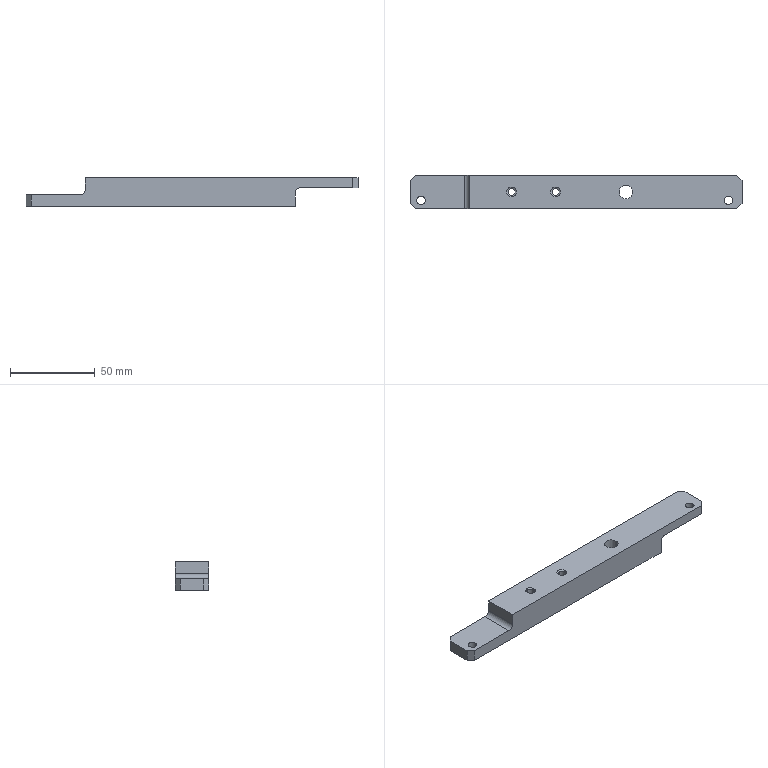Part | NX | 1 solid | 34 faces | box 196 x 20 x 17 mm | volume 49787 mm3 | plane 14 | cylinder 14 | cone 6 | commonest cylinder face diameters 4.2 x6 5 x4 6 x2 8 x2
STEP:
#1=CARTESIAN_POINT('',(-95.,10.,-1.5));
#2=VERTEX_POINT('',#1);
#3=CARTESIAN_POINT('',(-66.,10.,-1.5));
#4=VERTEX_POINT('',#3);
#5=CARTESIAN_POINT('',(0.,10.,-1.5));
#6=DIRECTION('',(1.,0.,0.));
#7=VECTOR('',#6,1000.);
#8=LINE('',#5,#7);
#9=EDGE_CURVE('',#2,#4,#8,.T.);
#10=ORIENTED_EDGE('',*,*,#9,.F.);
#11=CARTESIAN_POINT('',(-98.,7.,-1.5));
#12=VERTEX_POINT('',#11);
#13=CARTESIAN_POINT('',(-95.,10.,-1.5));
#14=DIRECTION('',(-0.7071,-0.7071,0.));
#15=VECTOR('',#14,1000.);
#16=LINE('',#13,#15);
#17=EDGE_CURVE('',#2,#12,#16,.T.);
#18=ORIENTED_EDGE('',*,*,#17,.T.);
#19=CARTESIAN_POINT('',(-98.,-7.,-1.5));
#20=VERTEX_POINT('',#19);
#21=CARTESIAN_POINT('',(-98.,-7.,-1.5));
#22=DIRECTION('',(0.,1.,0.));
#23=VECTOR('',#22,1000.);
#24=LINE('',#21,#23);
#25=EDGE_CURVE('',#20,#12,#24,.T.);
#26=ORIENTED_EDGE('',*,*,#25,.F.);
#27=CARTESIAN_POINT('',(-95.,-10.,-1.5));
#28=VERTEX_POINT('',#27);
#29=CARTESIAN_POINT('',(-98.,-7.,-1.5));
#30=DIRECTION('',(0.7071,-0.7071,0.));
#31=VECTOR('',#30,1000.);
#32=LINE('',#29,#31);
#33=EDGE_CURVE('',#20,#28,#32,.T.);
#34=ORIENTED_EDGE('',*,*,#33,.T.);
#35=CARTESIAN_POINT('',(-66.,-10.,-1.5));
#36=VERTEX_POINT('',#35);
#37=CARTESIAN_POINT('',(-66.,-10.,-1.5));
#38=DIRECTION('',(-1.,0.,0.));
#39=VECTOR('',#38,1000.);
#40=LINE('',#37,#39);
#41=EDGE_CURVE('',#36,#28,#40,.T.);
#42=ORIENTED_EDGE('',*,*,#41,.F.);
#43=CARTESIAN_POINT('',(-66.,10.,-1.5));
#44=DIRECTION('',(0.,-1.,0.));
#45=VECTOR('',#44,1000.);
#46=LINE('',#43,#45);
#47=EDGE_CURVE('',#4,#36,#46,.T.);
#48=ORIENTED_EDGE('',*,*,#47,.F.);
#49=EDGE_LOOP('',(#10,#18,#26,#34,#42,#48));
#50=FACE_BOUND('',#49,.T.);
#51=CARTESIAN_POINT('',(-94.,-5.,-1.5));
#52=VERTEX_POINT('',#51);
#53=CARTESIAN_POINT('',(-89.,-5.,-1.5));
#54=VERTEX_POINT('',#53);
#55=CARTESIAN_POINT('',(-91.5,-5.,-1.5));
#56=DIRECTION('',(0.,0.,-1.));
#57=DIRECTION('',(-1.,0.,0.));
#58=AXIS2_PLACEMENT_3D('',#55,#56,#57);
#59=CIRCLE('',#58,2.5);
#60=EDGE_CURVE('',#52,#54,#59,.T.);
#61=ORIENTED_EDGE('',*,*,#60,.T.);
#62=CARTESIAN_POINT('',(-91.5,-5.,-1.5));
#63=DIRECTION('',(0.,0.,-1.));
#64=DIRECTION('',(-1.,0.,0.));
#65=AXIS2_PLACEMENT_3D('',#62,#63,#64);
#66=CIRCLE('',#65,2.5);
#67=EDGE_CURVE('',#54,#52,#66,.T.);
#68=ORIENTED_EDGE('',*,*,#67,.T.);
#69=EDGE_LOOP('',(#61,#68));
#70=FACE_BOUND('',#69,.T.);
#71=CARTESIAN_POINT('',(-98.,10.,-1.5));
#72=DIRECTION('',(0.,0.,1.));
#73=DIRECTION('',(1.,0.,0.));
#74=AXIS2_PLACEMENT_3D('',#71,#72,#73);
#75=PLANE('',#74);
#76=ADVANCED_FACE('',(#50,#70),#75,.T.);
#77=CARTESIAN_POINT('',(61.,-10.,-0.5));
#78=VERTEX_POINT('',#77);
#79=CARTESIAN_POINT('',(64.,-10.,2.5));
#80=VERTEX_POINT('',#79);
#81=CARTESIAN_POINT('',(64.,-10.,-0.5));
#82=DIRECTION('',(0.,1.,0.));
#83=DIRECTION('',(-1.,0.,0.));
#84=AXIS2_PLACEMENT_3D('',#81,#82,#83);
#85=CIRCLE('',#84,3.);
#86=EDGE_CURVE('',#78,#80,#85,.T.);
#87=ORIENTED_EDGE('',*,*,#86,.T.);
#88=CARTESIAN_POINT('',(95.,-10.,2.5));
#89=VERTEX_POINT('',#88);
#90=CARTESIAN_POINT('',(64.,-10.,2.5));
#91=DIRECTION('',(1.,0.,0.));
#92=VECTOR('',#91,1000.);
#93=LINE('',#90,#92);
#94=EDGE_CURVE('',#80,#89,#93,.T.);
#95=ORIENTED_EDGE('',*,*,#94,.T.);
#96=CARTESIAN_POINT('',(95.,-10.,8.5));
#97=VERTEX_POINT('',#96);
#98=CARTESIAN_POINT('',(95.,-10.,2.5));
#99=DIRECTION('',(0.,0.,1.));
#100=VECTOR('',#99,1000.);
#101=LINE('',#98,#100);
#102=EDGE_CURVE('',#89,#97,#101,.T.);
#103=ORIENTED_EDGE('',*,*,#102,.T.);
#104=CARTESIAN_POINT('',(-63.,-10.,8.5));
#105=VERTEX_POINT('',#104);
#106=CARTESIAN_POINT('',(0.,-10.,8.5));
#107=DIRECTION('',(1.,0.,0.));
#108=VECTOR('',#107,1000.);
#109=LINE('',#106,#108);
#110=EDGE_CURVE('',#105,#97,#109,.T.);
#111=ORIENTED_EDGE('',*,*,#110,.F.);
#112=CARTESIAN_POINT('',(-63.,-10.,1.5));
#113=VERTEX_POINT('',#112);
#114=CARTESIAN_POINT('',(-63.,-10.,1.5));
#115=DIRECTION('',(0.,0.,1.));
#116=VECTOR('',#115,1000.);
#117=LINE('',#114,#116);
#118=EDGE_CURVE('',#113,#105,#117,.T.);
#119=ORIENTED_EDGE('',*,*,#118,.F.);
#120=CARTESIAN_POINT('',(-66.,-10.,1.5));
#121=DIRECTION('',(0.,1.,0.));
#122=DIRECTION('',(1.,0.,0.));
#123=AXIS2_PLACEMENT_3D('',#120,#121,#122);
#124=CIRCLE('',#123,3.);
#125=EDGE_CURVE('',#113,#36,#124,.T.);
#126=ORIENTED_EDGE('',*,*,#125,.T.);
#127=ORIENTED_EDGE('',*,*,#41,.T.);
#128=CARTESIAN_POINT('',(-95.,-10.,-8.5));
#129=VERTEX_POINT('',#128);
#130=CARTESIAN_POINT('',(-95.,-10.,-8.5));
#131=DIRECTION('',(0.,0.,1.));
#132=VECTOR('',#131,1000.);
#133=LINE('',#130,#132);
#134=EDGE_CURVE('',#129,#28,#133,.T.);
#135=ORIENTED_EDGE('',*,*,#134,.F.);
#136=CARTESIAN_POINT('',(61.,-10.,-8.5));
#137=VERTEX_POINT('',#136);
#138=CARTESIAN_POINT('',(0.,-10.,-8.5));
#139=DIRECTION('',(1.,0.,0.));
#140=VECTOR('',#139,1000.);
#141=LINE('',#138,#140);
#142=EDGE_CURVE('',#129,#137,#141,.T.);
#143=ORIENTED_EDGE('',*,*,#142,.T.);
#144=CARTESIAN_POINT('',(61.,-10.,-0.5));
#145=DIRECTION('',(0.,0.,-1.));
#146=VECTOR('',#145,1000.);
#147=LINE('',#144,#146);
#148=EDGE_CURVE('',#78,#137,#147,.T.);
#149=ORIENTED_EDGE('',*,*,#148,.F.);
#150=EDGE_LOOP('',(#87,#95,#103,#111,#119,#126,#127,#135,#143,#149));
#151=FACE_BOUND('',#150,.T.);
#152=CARTESIAN_POINT('',(-98.,-10.,8.5));
#153=DIRECTION('',(0.,1.,0.));
#154=DIRECTION('',(1.,0.,0.));
#155=AXIS2_PLACEMENT_3D('',#152,#153,#154);
#156=PLANE('',#155);
#157=ADVANCED_FACE('',(#151),#156,.F.);
#158=ORIENTED_EDGE('',*,*,#148,.T.);
#159=CARTESIAN_POINT('',(61.,10.,-8.5));
#160=VERTEX_POINT('',#159);
#161=CARTESIAN_POINT('',(61.,0.,-8.5));
#162=DIRECTION('',(0.,-1.,0.));
#163=VECTOR('',#162,1000.);
#164=LINE('',#161,#163);
#165=EDGE_CURVE('',#160,#137,#164,.T.);
#166=ORIENTED_EDGE('',*,*,#165,.F.);
#167=CARTESIAN_POINT('',(61.,10.,-0.5));
#168=VERTEX_POINT('',#167);
#169=CARTESIAN_POINT('',(61.,10.,0.));
#170=DIRECTION('',(0.,0.,-1.));
#171=VECTOR('',#170,1000.);
#172=LINE('',#169,#171);
#173=EDGE_CURVE('',#168,#160,#172,.T.);
#174=ORIENTED_EDGE('',*,*,#173,.F.);
#175=CARTESIAN_POINT('',(61.,10.339,-0.5));
#176=DIRECTION('',(0.,-1.,0.));
#177=VECTOR('',#176,1000.);
#178=LINE('',#175,#177);
#179=EDGE_CURVE('',#168,#78,#178,.T.);
#180=ORIENTED_EDGE('',*,*,#179,.T.);
#181=EDGE_LOOP('',(#158,#166,#174,#180));
#182=FACE_BOUND('',#181,.T.);
#183=CARTESIAN_POINT('',(61.,10.,2.5));
#184=DIRECTION('',(1.,0.,0.));
#185=DIRECTION('',(0.,1.,0.));
#186=AXIS2_PLACEMENT_3D('',#183,#184,#185);
#187=PLANE('',#186);
#188=ADVANCED_FACE('',(#182),#187,.T.);
#189=CARTESIAN_POINT('',(64.,10.,2.5));
#190=VERTEX_POINT('',#189);
#191=CARTESIAN_POINT('',(64.,10.,-0.5));
#192=DIRECTION('',(0.,-1.,0.));
#193=DIRECTION('',(-1.,0.,0.));
#194=AXIS2_PLACEMENT_3D('',#191,#192,#193);
#195=CIRCLE('',#194,3.);
#196=EDGE_CURVE('',#190,#168,#195,.T.);
#197=ORIENTED_EDGE('',*,*,#196,.F.);
#198=CARTESIAN_POINT('',(64.,10.,2.5));
#199=DIRECTION('',(0.,-1.,0.));
#200=VECTOR('',#199,1000.);
#201=LINE('',#198,#200);
#202=EDGE_CURVE('',#190,#80,#201,.T.);
#203=ORIENTED_EDGE('',*,*,#202,.T.);
#204=ORIENTED_EDGE('',*,*,#86,.F.);
#205=ORIENTED_EDGE('',*,*,#179,.F.);
#206=EDGE_LOOP('',(#197,#203,#204,#205));
#207=FACE_BOUND('',#206,.T.);
#208=CARTESIAN_POINT('',(64.,10.339,-0.5));
#209=DIRECTION('',(0.,-1.,0.));
#210=DIRECTION('',(-1.,0.,0.));
#211=AXIS2_PLACEMENT_3D('',#208,#209,#210);
#212=CYLINDRICAL_SURFACE('',#211,3.);
#213=ADVANCED_FACE('',(#207),#212,.F.);
#214=ORIENTED_EDGE('',*,*,#196,.T.);
#215=ORIENTED_EDGE('',*,*,#173,.T.);
#216=CARTESIAN_POINT('',(-95.,10.,-8.5));
#217=VERTEX_POINT('',#216);
#218=CARTESIAN_POINT('',(0.,10.,-8.5));
#219=DIRECTION('',(-1.,0.,0.));
#220=VECTOR('',#219,1000.);
#221=LINE('',#218,#220);
#222=EDGE_CURVE('',#160,#217,#221,.T.);
#223=ORIENTED_EDGE('',*,*,#222,.T.);
#224=CARTESIAN_POINT('',(-95.,10.,0.));
#225=DIRECTION('',(0.,0.,-1.));
#226=VECTOR('',#225,1000.);
#227=LINE('',#224,#226);
#228=EDGE_CURVE('',#2,#217,#227,.T.);
#229=ORIENTED_EDGE('',*,*,#228,.F.);
#230=ORIENTED_EDGE('',*,*,#9,.T.);
#231=CARTESIAN_POINT('',(-63.,10.,1.5));
#232=VERTEX_POINT('',#231);
#233=CARTESIAN_POINT('',(-66.,10.,1.5));
#234=DIRECTION('',(0.,-1.,0.));
#235=DIRECTION('',(1.,0.,0.));
#236=AXIS2_PLACEMENT_3D('',#233,#234,#235);
#237=CIRCLE('',#236,3.);
#238=EDGE_CURVE('',#4,#232,#237,.T.);
#239=ORIENTED_EDGE('',*,*,#238,.T.);
#240=CARTESIAN_POINT('',(-63.,10.,8.5));
#241=VERTEX_POINT('',#240);
#242=CARTESIAN_POINT('',(-63.,10.,0.));
#243=DIRECTION('',(0.,0.,1.));
#244=VECTOR('',#243,1000.);
#245=LINE('',#242,#244);
#246=EDGE_CURVE('',#232,#241,#245,.T.);
#247=ORIENTED_EDGE('',*,*,#246,.T.);
#248=CARTESIAN_POINT('',(95.,10.,8.5));
#249=VERTEX_POINT('',#248);
#250=CARTESIAN_POINT('',(0.,10.,8.5));
#251=DIRECTION('',(1.,0.,0.));
#252=VECTOR('',#251,1000.);
#253=LINE('',#250,#252);
#254=EDGE_CURVE('',#241,#249,#253,.T.);
#255=ORIENTED_EDGE('',*,*,#254,.T.);
#256=CARTESIAN_POINT('',(95.,10.,2.5));
#257=VERTEX_POINT('',#256);
#258=CARTESIAN_POINT('',(95.,10.,0.));
#259=DIRECTION('',(0.,0.,1.));
#260=VECTOR('',#259,1000.);
#261=LINE('',#258,#260);
#262=EDGE_CURVE('',#257,#249,#261,.T.);
#263=ORIENTED_EDGE('',*,*,#262,.F.);
#264=CARTESIAN_POINT('',(0.,10.,2.5));
#265=DIRECTION('',(-1.,0.,0.));
#266=VECTOR('',#265,1000.);
#267=LINE('',#264,#266);
#268=EDGE_CURVE('',#257,#190,#267,.T.);
#269=ORIENTED_EDGE('',*,*,#268,.T.);
#270=EDGE_LOOP('',(#214,#215,#223,#229,#230,#239,#247,#255,#263,#269));
#271=FACE_BOUND('',#270,.T.);
#272=CARTESIAN_POINT('',(29.5,10.,2.86));
#273=VERTEX_POINT('',#272);
#274=CARTESIAN_POINT('',(29.5,10.,-2.86));
#275=VERTEX_POINT('',#274);
#276=CARTESIAN_POINT('',(29.5,10.,0.));
#277=DIRECTION('',(0.,1.,0.));
#278=DIRECTION('',(0.,0.,-1.));
#279=AXIS2_PLACEMENT_3D('',#276,#277,#278);
#280=CIRCLE('',#279,2.86);
#281=EDGE_CURVE('',#273,#275,#280,.T.);
#282=ORIENTED_EDGE('',*,*,#281,.F.);
#283=CARTESIAN_POINT('',(29.5,10.,0.));
#284=DIRECTION('',(0.,1.,0.));
#285=DIRECTION('',(0.,0.,-1.));
#286=AXIS2_PLACEMENT_3D('',#283,#284,#285);
#287=CIRCLE('',#286,2.86);
#288=EDGE_CURVE('',#275,#273,#287,.T.);
#289=ORIENTED_EDGE('',*,*,#288,.F.);
#290=EDGE_LOOP('',(#282,#289));
#291=FACE_BOUND('',#290,.T.);
#292=CARTESIAN_POINT('',(98.,10.,8.5));
#293=DIRECTION('',(0.,-1.,0.));
#294=DIRECTION('',(0.,0.,-1.));
#295=AXIS2_PLACEMENT_3D('',#292,#293,#294);
#296=PLANE('',#295);
#297=ADVANCED_FACE('',(#271,#291),#296,.F.);
#298=ORIENTED_EDGE('',*,*,#268,.F.);
#299=CARTESIAN_POINT('',(98.,7.,2.5));
#300=VERTEX_POINT('',#299);
#301=CARTESIAN_POINT('',(95.,10.,2.5));
#302=DIRECTION('',(0.7071,-0.7071,0.));
#303=VECTOR('',#302,1000.);
#304=LINE('',#301,#303);
#305=EDGE_CURVE('',#257,#300,#304,.T.);
#306=ORIENTED_EDGE('',*,*,#305,.T.);
#307=CARTESIAN_POINT('',(98.,-7.,2.5));
#308=VERTEX_POINT('',#307);
#309=CARTESIAN_POINT('',(98.,7.,2.5));
#310=DIRECTION('',(0.,-1.,0.));
#311=VECTOR('',#310,1000.);
#312=LINE('',#309,#311);
#313=EDGE_CURVE('',#300,#308,#312,.T.);
#314=ORIENTED_EDGE('',*,*,#313,.T.);
#315=CARTESIAN_POINT('',(98.,-7.,2.5));
#316=DIRECTION('',(-0.7071,-0.7071,0.));
#317=VECTOR('',#316,1000.);
#318=LINE('',#315,#317);
#319=EDGE_CURVE('',#308,#89,#318,.T.);
#320=ORIENTED_EDGE('',*,*,#319,.T.);
#321=ORIENTED_EDGE('',*,*,#94,.F.);
#322=ORIENTED_EDGE('',*,*,#202,.F.);
#323=EDGE_LOOP('',(#298,#306,#314,#320,#321,#322));
#324=FACE_BOUND('',#323,.T.);
#325=CARTESIAN_POINT('',(92.5,-5.,2.5));
#326=VERTEX_POINT('',#325);
#327=CARTESIAN_POINT('',(87.5,-5.,2.5));
#328=VERTEX_POINT('',#327);
#329=CARTESIAN_POINT('',(90.,-5.,2.5));
#330=DIRECTION('',(0.,0.,1.));
#331=DIRECTION('',(1.,0.,0.));
#332=AXIS2_PLACEMENT_3D('',#329,#330,#331);
#333=CIRCLE('',#332,2.5);
#334=EDGE_CURVE('',#326,#328,#333,.T.);
#335=ORIENTED_EDGE('',*,*,#334,.T.);
#336=CARTESIAN_POINT('',(90.,-5.,2.5));
#337=DIRECTION('',(0.,0.,1.));
#338=DIRECTION('',(1.,0.,0.));
#339=AXIS2_PLACEMENT_3D('',#336,#337,#338);
#340=CIRCLE('',#339,2.5);
#341=EDGE_CURVE('',#328,#326,#340,.T.);
#342=ORIENTED_EDGE('',*,*,#341,.T.);
#343=EDGE_LOOP('',(#335,#342));
#344=FACE_BOUND('',#343,.T.);
#345=CARTESIAN_POINT('',(98.,10.,2.5));
#346=DIRECTION('',(0.,0.,-1.));
#347=DIRECTION('',(0.,-1.,0.));
#348=AXIS2_PLACEMENT_3D('',#345,#346,#347);
#349=PLANE('',#348);
#350=ADVANCED_FACE('',(#324,#344),#349,.T.);
#351=CARTESIAN_POINT('',(98.,7.,8.5));
#352=VERTEX_POINT('',#351);
#353=CARTESIAN_POINT('',(105.,0.,8.5));
#354=DIRECTION('',(-0.7071,0.7071,0.));
#355=VECTOR('',#354,1000.);
#356=LINE('',#353,#355);
#357=EDGE_CURVE('',#352,#249,#356,.T.);
#358=ORIENTED_EDGE('',*,*,#357,.F.);
#359=CARTESIAN_POINT('',(98.,7.,2.5));
#360=DIRECTION('',(0.,0.,1.));
#361=VECTOR('',#360,1000.);
#362=LINE('',#359,#361);
#363=EDGE_CURVE('',#300,#352,#362,.T.);
#364=ORIENTED_EDGE('',*,*,#363,.F.);
#365=ORIENTED_EDGE('',*,*,#305,.F.);
#366=ORIENTED_EDGE('',*,*,#262,.T.);
#367=EDGE_LOOP('',(#358,#364,#365,#366));
#368=FACE_BOUND('',#367,.T.);
#369=CARTESIAN_POINT('',(95.,10.,8.5));
#370=DIRECTION('',(-0.7071,-0.7071,0.));
#371=DIRECTION('',(-0.7071,0.7071,0.));
#372=AXIS2_PLACEMENT_3D('',#369,#370,#371);
#373=PLANE('',#372);
#374=ADVANCED_FACE('',(#368),#373,.F.);
#375=ORIENTED_EDGE('',*,*,#313,.F.);
#376=ORIENTED_EDGE('',*,*,#363,.T.);
#377=CARTESIAN_POINT('',(98.,-7.,8.5));
#378=VERTEX_POINT('',#377);
#379=CARTESIAN_POINT('',(98.,0.,8.5));
#380=DIRECTION('',(0.,1.,0.));
#381=VECTOR('',#380,1000.);
#382=LINE('',#379,#381);
#383=EDGE_CURVE('',#378,#352,#382,.T.);
#384=ORIENTED_EDGE('',*,*,#383,.F.);
#385=CARTESIAN_POINT('',(98.,-7.,2.5));
#386=DIRECTION('',(0.,0.,1.));
#387=VECTOR('',#386,1000.);
#388=LINE('',#385,#387);
#389=EDGE_CURVE('',#308,#378,#388,.T.);
#390=ORIENTED_EDGE('',*,*,#389,.F.);
#391=EDGE_LOOP('',(#375,#376,#384,#390));
#392=FACE_BOUND('',#391,.T.);
#393=CARTESIAN_POINT('',(98.,-10.,8.5));
#394=DIRECTION('',(-1.,0.,0.));
#395=DIRECTION('',(0.,0.,1.));
#396=AXIS2_PLACEMENT_3D('',#393,#394,#395);
#397=PLANE('',#396);
#398=ADVANCED_FACE('',(#392),#397,.F.);
#399=CARTESIAN_POINT('',(105.,0.,8.5));
#400=DIRECTION('',(0.7071,0.7071,0.));
#401=VECTOR('',#400,1000.);
#402=LINE('',#399,#401);
#403=EDGE_CURVE('',#97,#378,#402,.T.);
#404=ORIENTED_EDGE('',*,*,#403,.F.);
#405=ORIENTED_EDGE('',*,*,#102,.F.);
#406=ORIENTED_EDGE('',*,*,#319,.F.);
#407=ORIENTED_EDGE('',*,*,#389,.T.);
#408=EDGE_LOOP('',(#404,#405,#406,#407));
#409=FACE_BOUND('',#408,.T.);
#410=CARTESIAN_POINT('',(98.,-7.,8.5));
#411=DIRECTION('',(-0.7071,0.7071,0.));
#412=DIRECTION('',(0.,0.,1.));
#413=AXIS2_PLACEMENT_3D('',#410,#411,#412);
#414=PLANE('',#413);
#415=ADVANCED_FACE('',(#409),#414,.F.);
#416=CARTESIAN_POINT('',(87.5,-5.,8.5));
#417=VERTEX_POINT('',#416);
#418=CARTESIAN_POINT('',(92.5,-5.,8.5));
#419=VERTEX_POINT('',#418);
#420=CARTESIAN_POINT('',(90.,-5.,8.5));
#421=DIRECTION('',(0.,0.,1.));
#422=DIRECTION('',(1.,0.,0.));
#423=AXIS2_PLACEMENT_3D('',#420,#421,#422);
#424=CIRCLE('',#423,2.5);
#425=EDGE_CURVE('',#417,#419,#424,.T.);
#426=ORIENTED_EDGE('',*,*,#425,.T.);
#427=CARTESIAN_POINT('',(92.5,-5.,-8.5));
#428=DIRECTION('',(0.,0.,1.));
#429=VECTOR('',#428,1000.);
#430=LINE('',#427,#429);
#431=EDGE_CURVE('',#326,#419,#430,.T.);
#432=ORIENTED_EDGE('',*,*,#431,.F.);
#433=ORIENTED_EDGE('',*,*,#341,.F.);
#434=CARTESIAN_POINT('',(87.5,-5.,-8.5));
#435=DIRECTION('',(0.,0.,1.));
#436=VECTOR('',#435,1000.);
#437=LINE('',#434,#436);
#438=EDGE_CURVE('',#328,#417,#437,.T.);
#439=ORIENTED_EDGE('',*,*,#438,.T.);
#440=EDGE_LOOP('',(#426,#432,#433,#439));
#441=FACE_BOUND('',#440,.T.);
#442=CARTESIAN_POINT('',(90.,-5.,-8.5));
#443=DIRECTION('',(0.,0.,1.));
#444=DIRECTION('',(1.,0.,0.));
#445=AXIS2_PLACEMENT_3D('',#442,#443,#444);
#446=CYLINDRICAL_SURFACE('',#445,2.5);
#447=ADVANCED_FACE('',(#441),#446,.F.);
#448=CARTESIAN_POINT('',(-9.14,0.,8.5));
#449=VERTEX_POINT('',#448);
#450=CARTESIAN_POINT('',(-14.86,0.,8.5));
#451=VERTEX_POINT('',#450);
#452=CARTESIAN_POINT('',(-12.,0.,8.5));
#453=DIRECTION('',(0.,0.,1.));
#454=DIRECTION('',(1.,0.,0.));
#455=AXIS2_PLACEMENT_3D('',#452,#453,#454);
#456=CIRCLE('',#455,2.86);
#457=EDGE_CURVE('',#449,#451,#456,.T.);
#458=ORIENTED_EDGE('',*,*,#457,.T.);
#459=CARTESIAN_POINT('',(-14.1,0.,8.061));
#460=VERTEX_POINT('',#459);
#461=CARTESIAN_POINT('',(-14.1,0.,8.061));
#462=DIRECTION('',(-0.866,0.,0.5));
#463=VECTOR('',#462,1000.);
#464=LINE('',#461,#463);
#465=EDGE_CURVE('',#451,#460,#464,.F.);
#466=ORIENTED_EDGE('',*,*,#465,.T.);
#467=CARTESIAN_POINT('',(-12.066,2.099,8.061));
#468=VERTEX_POINT('',#467);
#469=CARTESIAN_POINT('',(-12.,0.,8.061));
#470=DIRECTION('',(0.,0.,1.));
#471=DIRECTION('',(1.,0.,0.));
#472=AXIS2_PLACEMENT_3D('',#469,#470,#471);
#473=CIRCLE('',#472,2.1);
#474=EDGE_CURVE('',#468,#460,#473,.T.);
#475=ORIENTED_EDGE('',*,*,#474,.F.);
#476=CARTESIAN_POINT('',(-9.9,0.,8.061));
#477=VERTEX_POINT('',#476);
#478=CARTESIAN_POINT('',(-12.,0.,8.061));
#479=DIRECTION('',(0.,0.,1.));
#480=DIRECTION('',(1.,0.,0.));
#481=AXIS2_PLACEMENT_3D('',#478,#479,#480);
#482=CIRCLE('',#481,2.1);
#483=EDGE_CURVE('',#477,#468,#482,.T.);
#484=ORIENTED_EDGE('',*,*,#483,.F.);
#485=CARTESIAN_POINT('',(-9.9,0.,8.061));
#486=DIRECTION('',(0.866,0.,0.5));
#487=VECTOR('',#486,1000.);
#488=LINE('',#485,#487);
#489=EDGE_CURVE('',#449,#477,#488,.F.);
#490=ORIENTED_EDGE('',*,*,#489,.F.);
#491=EDGE_LOOP('',(#458,#466,#475,#484,#490));
#492=FACE_BOUND('',#491,.T.);
#493=CARTESIAN_POINT('',(-12.,0.,8.061));
#494=DIRECTION('',(0.,0.,1.));
#495=DIRECTION('',(1.,0.,0.));
#496=AXIS2_PLACEMENT_3D('',#493,#494,#495);
#497=CONICAL_SURFACE('',#496,2.1,1.047);
#498=ADVANCED_FACE('',(#492),#497,.F.);
#499=ORIENTED_EDGE('',*,*,#403,.T.);
#500=ORIENTED_EDGE('',*,*,#383,.T.);
#501=ORIENTED_EDGE('',*,*,#357,.T.);
#502=ORIENTED_EDGE('',*,*,#254,.F.);
#503=CARTESIAN_POINT('',(-63.,0.,8.5));
#504=DIRECTION('',(0.,1.,0.));
#505=VECTOR('',#504,1000.);
#506=LINE('',#503,#505);
#507=EDGE_CURVE('',#105,#241,#506,.T.);
#508=ORIENTED_EDGE('',*,*,#507,.F.);
#509=ORIENTED_EDGE('',*,*,#110,.T.);
#510=EDGE_LOOP('',(#499,#500,#501,#502,#508,#509));
#511=FACE_BOUND('',#510,.T.);
#512=ORIENTED_EDGE('',*,*,#425,.F.);
#513=CARTESIAN_POINT('',(90.,-5.,8.5));
#514=DIRECTION('',(0.,0.,1.));
#515=DIRECTION('',(1.,0.,0.));
#516=AXIS2_PLACEMENT_3D('',#513,#514,#515);
#517=CIRCLE('',#516,2.5);
#518=EDGE_CURVE('',#419,#417,#517,.T.);
#519=ORIENTED_EDGE('',*,*,#518,.F.);
#520=EDGE_LOOP('',(#512,#519));
#521=FACE_BOUND('',#520,.T.);
#522=CARTESIAN_POINT('',(-40.86,0.,8.5));
#523=VERTEX_POINT('',#522);
#524=CARTESIAN_POINT('',(-35.14,0.,8.5));
#525=VERTEX_POINT('',#524);
#526=CARTESIAN_POINT('',(-38.,0.,8.5));
#527=DIRECTION('',(0.,0.,1.));
#528=DIRECTION('',(1.,0.,0.));
#529=AXIS2_PLACEMENT_3D('',#526,#527,#528);
#530=CIRCLE('',#529,2.86);
#531=EDGE_CURVE('',#523,#525,#530,.T.);
#532=ORIENTED_EDGE('',*,*,#531,.F.);
#533=CARTESIAN_POINT('',(-38.,0.,8.5));
#534=DIRECTION('',(0.,0.,1.));
#535=DIRECTION('',(1.,0.,0.));
#536=AXIS2_PLACEMENT_3D('',#533,#534,#535);
#537=CIRCLE('',#536,2.86);
#538=EDGE_CURVE('',#525,#523,#537,.T.);
#539=ORIENTED_EDGE('',*,*,#538,.F.);
#540=EDGE_LOOP('',(#532,#539));
#541=FACE_BOUND('',#540,.T.);
#542=CARTESIAN_POINT('',(33.5,0.,8.5));
#543=VERTEX_POINT('',#542);
#544=CARTESIAN_POINT('',(25.5,0.,8.5));
#545=VERTEX_POINT('',#544);
#546=CARTESIAN_POINT('',(29.5,0.,8.5));
#547=DIRECTION('',(0.,0.,1.));
#548=DIRECTION('',(1.,0.,0.));
#549=AXIS2_PLACEMENT_3D('',#546,#547,#548);
#550=CIRCLE('',#549,4.);
#551=EDGE_CURVE('',#543,#545,#550,.T.);
#552=ORIENTED_EDGE('',*,*,#551,.F.);
#553=CARTESIAN_POINT('',(29.5,0.,8.5));
#554=DIRECTION('',(0.,0.,1.));
#555=DIRECTION('',(1.,0.,0.));
#556=AXIS2_PLACEMENT_3D('',#553,#554,#555);
#557=CIRCLE('',#556,4.);
#558=EDGE_CURVE('',#545,#543,#557,.T.);
#559=ORIENTED_EDGE('',*,*,#558,.F.);
#560=EDGE_LOOP('',(#552,#559));
#561=FACE_BOUND('',#560,.T.);
#562=ORIENTED_EDGE('',*,*,#457,.F.);
#563=CARTESIAN_POINT('',(-12.,0.,8.5));
#564=DIRECTION('',(0.,0.,1.));
#565=DIRECTION('',(1.,0.,0.));
#566=AXIS2_PLACEMENT_3D('',#563,#564,#565);
#567=CIRCLE('',#566,2.86);
#568=EDGE_CURVE('',#451,#449,#567,.T.);
#569=ORIENTED_EDGE('',*,*,#568,.F.);
#570=EDGE_LOOP('',(#562,#569));
#571=FACE_BOUND('',#570,.T.);
#572=CARTESIAN_POINT('',(0.,0.,8.5));
#573=DIRECTION('',(0.,0.,1.));
#574=DIRECTION('',(1.,0.,0.));
#575=AXIS2_PLACEMENT_3D('',#572,#573,#574);
#576=PLANE('',#575);
#577=ADVANCED_FACE('',(#511,#521,#541,#561,#571),#576,.T.);
#578=ORIENTED_EDGE('',*,*,#33,.F.);
#579=CARTESIAN_POINT('',(-98.,-7.,-8.5));
#580=VERTEX_POINT('',#579);
#581=CARTESIAN_POINT('',(-98.,-7.,-8.5));
#582=DIRECTION('',(0.,0.,1.));
#583=VECTOR('',#582,1000.);
#584=LINE('',#581,#583);
#585=EDGE_CURVE('',#580,#20,#584,.T.);
#586=ORIENTED_EDGE('',*,*,#585,.F.);
#587=CARTESIAN_POINT('',(-105.,0.,-8.5));
#588=DIRECTION('',(0.7071,-0.7071,0.));
#589=VECTOR('',#588,1000.);
#590=LINE('',#587,#589);
#591=EDGE_CURVE('',#580,#129,#590,.T.);
#592=ORIENTED_EDGE('',*,*,#591,.T.);
#593=ORIENTED_EDGE('',*,*,#134,.T.);
#594=EDGE_LOOP('',(#578,#586,#592,#593));
#595=FACE_BOUND('',#594,.T.);
#596=CARTESIAN_POINT('',(-95.,-10.,-1.5));
#597=DIRECTION('',(0.7071,0.7071,0.));
#598=DIRECTION('',(0.,0.,-1.));
#599=AXIS2_PLACEMENT_3D('',#596,#597,#598);
#600=PLANE('',#599);
#601=ADVANCED_FACE('',(#595),#600,.F.);
#602=ORIENTED_EDGE('',*,*,#591,.F.);
#603=CARTESIAN_POINT('',(-98.,7.,-8.5));
#604=VERTEX_POINT('',#603);
#605=CARTESIAN_POINT('',(-98.,0.,-8.5));
#606=DIRECTION('',(0.,-1.,0.));
#607=VECTOR('',#606,1000.);
#608=LINE('',#605,#607);
#609=EDGE_CURVE('',#604,#580,#608,.T.);
#610=ORIENTED_EDGE('',*,*,#609,.F.);
#611=CARTESIAN_POINT('',(-105.,0.,-8.5));
#612=DIRECTION('',(-0.7071,-0.7071,0.));
#613=VECTOR('',#612,1000.);
#614=LINE('',#611,#613);
#615=EDGE_CURVE('',#217,#604,#614,.T.);
#616=ORIENTED_EDGE('',*,*,#615,.F.);
#617=ORIENTED_EDGE('',*,*,#222,.F.);
#618=ORIENTED_EDGE('',*,*,#165,.T.);
#619=ORIENTED_EDGE('',*,*,#142,.F.);
#620=EDGE_LOOP('',(#602,#610,#616,#617,#618,#619));
#621=FACE_BOUND('',#620,.T.);
#622=CARTESIAN_POINT('',(25.5,0.,-8.5));
#623=VERTEX_POINT('',#622);
#624=CARTESIAN_POINT('',(33.5,0.,-8.5));
#625=VERTEX_POINT('',#624);
#626=CARTESIAN_POINT('',(29.5,0.,-8.5));
#627=DIRECTION('',(0.,0.,1.));
#628=DIRECTION('',(1.,0.,0.));
#629=AXIS2_PLACEMENT_3D('',#626,#627,#628);
#630=CIRCLE('',#629,4.);
#631=EDGE_CURVE('',#623,#625,#630,.T.);
#632=ORIENTED_EDGE('',*,*,#631,.T.);
#633=CARTESIAN_POINT('',(29.5,0.,-8.5));
#634=DIRECTION('',(0.,0.,1.));
#635=DIRECTION('',(1.,0.,0.));
#636=AXIS2_PLACEMENT_3D('',#633,#634,#635);
#637=CIRCLE('',#636,4.);
#638=EDGE_CURVE('',#625,#623,#637,.T.);
#639=ORIENTED_EDGE('',*,*,#638,.T.);
#640=EDGE_LOOP('',(#632,#639));
#641=FACE_BOUND('',#640,.T.);
#642=CARTESIAN_POINT('',(-11.934,-2.099,-8.5));
#643=VERTEX_POINT('',#642);
#644=CARTESIAN_POINT('',(-12.066,2.099,-8.5));
#645=VERTEX_POINT('',#644);
#646=CARTESIAN_POINT('',(-12.,0.,-8.5));
#647=DIRECTION('',(0.,0.,1.));
#648=DIRECTION('',(0.03164,-0.9995,0.));
#649=AXIS2_PLACEMENT_3D('',#646,#647,#648);
#650=CIRCLE('',#649,2.1);
#651=EDGE_CURVE('',#643,#645,#650,.T.);
#652=ORIENTED_EDGE('',*,*,#651,.T.);
#653=CARTESIAN_POINT('',(-12.,0.,-8.5));
#654=DIRECTION('',(0.,0.,1.));
#655=DIRECTION('',(0.03164,-0.9995,0.));
#656=AXIS2_PLACEMENT_3D('',#653,#654,#655);
#657=CIRCLE('',#656,2.1);
#658=EDGE_CURVE('',#645,#643,#657,.T.);
#659=ORIENTED_EDGE('',*,*,#658,.T.);
#660=EDGE_LOOP('',(#652,#659));
#661=FACE_BOUND('',#660,.T.);
#662=CARTESIAN_POINT('',(-94.,-5.,-8.5));
#663=VERTEX_POINT('',#662);
#664=CARTESIAN_POINT('',(-89.,-5.,-8.5));
#665=VERTEX_POINT('',#664);
#666=CARTESIAN_POINT('',(-91.5,-5.,-8.5));
#667=DIRECTION('',(0.,0.,1.));
#668=DIRECTION('',(1.,0.,0.));
#669=AXIS2_PLACEMENT_3D('',#666,#667,#668);
#670=CIRCLE('',#669,2.5);
#671=EDGE_CURVE('',#663,#665,#670,.T.);
#672=ORIENTED_EDGE('',*,*,#671,.T.);
#673=CARTESIAN_POINT('',(-91.5,-5.,-8.5));
#674=DIRECTION('',(0.,0.,1.));
#675=DIRECTION('',(1.,0.,0.));
#676=AXIS2_PLACEMENT_3D('',#673,#674,#675);
#677=CIRCLE('',#676,2.5);
#678=EDGE_CURVE('',#665,#663,#677,.T.);
#679=ORIENTED_EDGE('',*,*,#678,.T.);
#680=EDGE_LOOP('',(#672,#679));
#681=FACE_BOUND('',#680,.T.);
#682=CARTESIAN_POINT('',(-38.066,2.099,-8.5));
#683=VERTEX_POINT('',#682);
#684=CARTESIAN_POINT('',(-37.934,-2.099,-8.5));
#685=VERTEX_POINT('',#684);
#686=CARTESIAN_POINT('',(-38.,0.,-8.5));
#687=DIRECTION('',(0.,0.,1.));
#688=DIRECTION('',(0.03164,-0.9995,0.));
#689=AXIS2_PLACEMENT_3D('',#686,#687,#688);
#690=CIRCLE('',#689,2.1);
#691=EDGE_CURVE('',#683,#685,#690,.T.);
#692=ORIENTED_EDGE('',*,*,#691,.T.);
#693=CARTESIAN_POINT('',(-38.,0.,-8.5));
#694=DIRECTION('',(0.,0.,1.));
#695=DIRECTION('',(0.03164,-0.9995,0.));
#696=AXIS2_PLACEMENT_3D('',#693,#694,#695);
#697=CIRCLE('',#696,2.1);
#698=EDGE_CURVE('',#685,#683,#697,.T.);
#699=ORIENTED_EDGE('',*,*,#698,.T.);
#700=EDGE_LOOP('',(#692,#699));
#701=FACE_BOUND('',#700,.T.);
#702=CARTESIAN_POINT('',(0.,0.,-8.5));
#703=DIRECTION('',(0.,0.,1.));
#704=DIRECTION('',(1.,0.,0.));
#705=AXIS2_PLACEMENT_3D('',#702,#703,#704);
#706=PLANE('',#705);
#707=ADVANCED_FACE('',(#621,#641,#661,#681,#701),#706,.F.);
#708=ORIENTED_EDGE('',*,*,#238,.F.);
#709=ORIENTED_EDGE('',*,*,#47,.T.);
#710=ORIENTED_EDGE('',*,*,#125,.F.);
#711=CARTESIAN_POINT('',(-63.,10.339,1.5));
#712=DIRECTION('',(0.,-1.,0.));
#713=VECTOR('',#712,1000.);
#714=LINE('',#711,#713);
#715=EDGE_CURVE('',#232,#113,#714,.T.);
#716=ORIENTED_EDGE('',*,*,#715,.F.);
#717=EDGE_LOOP('',(#708,#709,#710,#716));
#718=FACE_BOUND('',#717,.T.);
#719=CARTESIAN_POINT('',(-66.,10.339,1.5));
#720=DIRECTION('',(0.,-1.,0.));
#721=DIRECTION('',(1.,0.,0.));
#722=AXIS2_PLACEMENT_3D('',#719,#720,#721);
#723=CYLINDRICAL_SURFACE('',#722,3.);
#724=ADVANCED_FACE('',(#718),#723,.F.);
#725=ORIENTED_EDGE('',*,*,#118,.T.);
#726=ORIENTED_EDGE('',*,*,#507,.T.);
#727=ORIENTED_EDGE('',*,*,#246,.F.);
#728=ORIENTED_EDGE('',*,*,#715,.T.);
#729=EDGE_LOOP('',(#725,#726,#727,#728));
#730=FACE_BOUND('',#729,.T.);
#731=CARTESIAN_POINT('',(-63.,10.,-1.5));
#732=DIRECTION('',(-1.,0.,0.));
#733=DIRECTION('',(0.,0.,1.));
#734=AXIS2_PLACEMENT_3D('',#731,#732,#733);
#735=PLANE('',#734);
#736=ADVANCED_FACE('',(#730),#735,.T.);
#737=ORIENTED_EDGE('',*,*,#17,.F.);
#738=ORIENTED_EDGE('',*,*,#228,.T.);
#739=ORIENTED_EDGE('',*,*,#615,.T.);
#740=CARTESIAN_POINT('',(-98.,7.,-8.5));
#741=DIRECTION('',(0.,0.,1.));
#742=VECTOR('',#741,1000.);
#743=LINE('',#740,#742);
#744=EDGE_CURVE('',#604,#12,#743,.T.);
#745=ORIENTED_EDGE('',*,*,#744,.T.);
#746=EDGE_LOOP('',(#737,#738,#739,#745));
#747=FACE_BOUND('',#746,.T.);
#748=CARTESIAN_POINT('',(-98.,7.,-1.5));
#749=DIRECTION('',(0.7071,-0.7071,0.));
#750=DIRECTION('',(0.,0.,-1.));
#751=AXIS2_PLACEMENT_3D('',#748,#749,#750);
#752=PLANE('',#751);
#753=ADVANCED_FACE('',(#747),#752,.F.);
#754=ORIENTED_EDGE('',*,*,#609,.T.);
#755=ORIENTED_EDGE('',*,*,#585,.T.);
#756=ORIENTED_EDGE('',*,*,#25,.T.);
#757=ORIENTED_EDGE('',*,*,#744,.F.);
#758=EDGE_LOOP('',(#754,#755,#756,#757));
#759=FACE_BOUND('',#758,.T.);
#760=CARTESIAN_POINT('',(-98.,10.,8.5));
#761=DIRECTION('',(1.,0.,0.));
#762=DIRECTION('',(0.,1.,0.));
#763=AXIS2_PLACEMENT_3D('',#760,#761,#762);
#764=PLANE('',#763);
#765=ADVANCED_FACE('',(#759),#764,.F.);
#766=ORIENTED_EDGE('',*,*,#60,.F.);
#767=CARTESIAN_POINT('',(-94.,-5.,-8.5));
#768=DIRECTION('',(0.,0.,1.));
#769=VECTOR('',#768,1000.);
#770=LINE('',#767,#769);
#771=EDGE_CURVE('',#52,#663,#770,.F.);
#772=ORIENTED_EDGE('',*,*,#771,.T.);
#773=ORIENTED_EDGE('',*,*,#678,.F.);
#774=CARTESIAN_POINT('',(-89.,-5.,-8.5));
#775=DIRECTION('',(0.,0.,1.));
#776=VECTOR('',#775,1000.);
#777=LINE('',#774,#776);
#778=EDGE_CURVE('',#54,#665,#777,.F.);
#779=ORIENTED_EDGE('',*,*,#778,.F.);
#780=EDGE_LOOP('',(#766,#772,#773,#779));
#781=FACE_BOUND('',#780,.T.);
#782=CARTESIAN_POINT('',(-91.5,-5.,-8.5));
#783=DIRECTION('',(0.,0.,1.));
#784=DIRECTION('',(1.,0.,0.));
#785=AXIS2_PLACEMENT_3D('',#782,#783,#784);
#786=CYLINDRICAL_SURFACE('',#785,2.5);
#787=ADVANCED_FACE('',(#781),#786,.F.);
#788=CARTESIAN_POINT('',(-11.934,-2.099,8.061));
#789=VERTEX_POINT('',#788);
#790=CARTESIAN_POINT('',(-12.,0.,8.061));
#791=DIRECTION('',(0.,0.,1.));
#792=DIRECTION('',(1.,0.,0.));
#793=AXIS2_PLACEMENT_3D('',#790,#791,#792);
#794=CIRCLE('',#793,2.1);
#795=EDGE_CURVE('',#460,#789,#794,.T.);
#796=ORIENTED_EDGE('',*,*,#795,.T.);
#797=CARTESIAN_POINT('',(-11.934,-2.099,0.));
#798=DIRECTION('',(0.,0.,1.));
#799=VECTOR('',#798,1000.);
#800=LINE('',#797,#799);
#801=EDGE_CURVE('',#643,#789,#800,.T.);
#802=ORIENTED_EDGE('',*,*,#801,.F.);
#803=ORIENTED_EDGE('',*,*,#658,.F.);
#804=CARTESIAN_POINT('',(-12.066,2.099,0.));
#805=DIRECTION('',(0.,0.,1.));
#806=VECTOR('',#805,1000.);
#807=LINE('',#804,#806);
#808=EDGE_CURVE('',#645,#468,#807,.T.);
#809=ORIENTED_EDGE('',*,*,#808,.T.);
#810=ORIENTED_EDGE('',*,*,#474,.T.);
#811=EDGE_LOOP('',(#796,#802,#803,#809,#810));
#812=FACE_BOUND('',#811,.T.);
#813=CARTESIAN_POINT('',(-12.,0.,0.));
#814=DIRECTION('',(0.,0.,1.));
#815=DIRECTION('',(0.03164,-0.9995,0.));
#816=AXIS2_PLACEMENT_3D('',#813,#814,#815);
#817=CYLINDRICAL_SURFACE('',#816,2.1);
#818=ADVANCED_FACE('',(#812),#817,.F.);
#819=ORIENTED_EDGE('',*,*,#631,.F.);
#820=CARTESIAN_POINT('',(25.5,0.,-8.5));
#821=DIRECTION('',(0.,0.,1.));
#822=VECTOR('',#821,1000.);
#823=LINE('',#820,#822);
#824=EDGE_CURVE('',#545,#623,#823,.F.);
#825=ORIENTED_EDGE('',*,*,#824,.F.);
#826=ORIENTED_EDGE('',*,*,#558,.T.);
#827=CARTESIAN_POINT('',(33.5,0.,-8.5));
#828=DIRECTION('',(0.,0.,1.));
#829=VECTOR('',#828,1000.);
#830=LINE('',#827,#829);
#831=EDGE_CURVE('',#543,#625,#830,.F.);
#832=ORIENTED_EDGE('',*,*,#831,.T.);
#833=EDGE_LOOP('',(#819,#825,#826,#832));
#834=FACE_BOUND('',#833,.T.);
#835=CARTESIAN_POINT('',(29.5,0.,-8.5));
#836=DIRECTION('',(0.,0.,1.));
#837=DIRECTION('',(1.,0.,0.));
#838=AXIS2_PLACEMENT_3D('',#835,#836,#837);
#839=CYLINDRICAL_SURFACE('',#838,4.);
#840=ADVANCED_FACE('',(#834),#839,.F.);
#841=CARTESIAN_POINT('',(-40.1,0.,8.061));
#842=VERTEX_POINT('',#841);
#843=CARTESIAN_POINT('',(-37.934,-2.099,8.061));
#844=VERTEX_POINT('',#843);
#845=CARTESIAN_POINT('',(-38.,0.,8.061));
#846=DIRECTION('',(0.,0.,1.));
#847=DIRECTION('',(1.,0.,0.));
#848=AXIS2_PLACEMENT_3D('',#845,#846,#847);
#849=CIRCLE('',#848,2.1);
#850=EDGE_CURVE('',#842,#844,#849,.T.);
#851=ORIENTED_EDGE('',*,*,#850,.T.);
#852=CARTESIAN_POINT('',(-37.934,-2.099,0.));
#853=DIRECTION('',(0.,0.,1.));
#854=VECTOR('',#853,1000.);
#855=LINE('',#852,#854);
#856=EDGE_CURVE('',#844,#685,#855,.F.);
#857=ORIENTED_EDGE('',*,*,#856,.T.);
#858=ORIENTED_EDGE('',*,*,#691,.F.);
#859=CARTESIAN_POINT('',(-38.066,2.099,8.061));
#860=VERTEX_POINT('',#859);
#861=CARTESIAN_POINT('',(-38.066,2.099,0.));
#862=DIRECTION('',(0.,0.,1.));
#863=VECTOR('',#862,1000.);
#864=LINE('',#861,#863);
#865=EDGE_CURVE('',#860,#683,#864,.F.);
#866=ORIENTED_EDGE('',*,*,#865,.F.);
#867=CARTESIAN_POINT('',(-38.,0.,8.061));
#868=DIRECTION('',(0.,0.,1.));
#869=DIRECTION('',(1.,0.,0.));
#870=AXIS2_PLACEMENT_3D('',#867,#868,#869);
#871=CIRCLE('',#870,2.1);
#872=EDGE_CURVE('',#860,#842,#871,.T.);
#873=ORIENTED_EDGE('',*,*,#872,.T.);
#874=EDGE_LOOP('',(#851,#857,#858,#866,#873));
#875=FACE_BOUND('',#874,.T.);
#876=CARTESIAN_POINT('',(-38.,0.,0.));
#877=DIRECTION('',(0.,0.,1.));
#878=DIRECTION('',(0.03164,-0.9995,0.));
#879=AXIS2_PLACEMENT_3D('',#876,#877,#878);
#880=CYLINDRICAL_SURFACE('',#879,2.1);
#881=ADVANCED_FACE('',(#875),#880,.F.);
#882=ORIENTED_EDGE('',*,*,#531,.T.);
#883=CARTESIAN_POINT('',(-35.9,0.,8.061));
#884=VERTEX_POINT('',#883);
#885=CARTESIAN_POINT('',(-35.14,0.,8.5));
#886=DIRECTION('',(0.866,0.,0.5));
#887=VECTOR('',#886,1000.);
#888=LINE('',#885,#887);
#889=EDGE_CURVE('',#884,#525,#888,.T.);
#890=ORIENTED_EDGE('',*,*,#889,.F.);
#891=CARTESIAN_POINT('',(-38.,0.,8.061));
#892=DIRECTION('',(0.,0.,1.));
#893=DIRECTION('',(1.,0.,0.));
#894=AXIS2_PLACEMENT_3D('',#891,#892,#893);
#895=CIRCLE('',#894,2.1);
#896=EDGE_CURVE('',#844,#884,#895,.T.);
#897=ORIENTED_EDGE('',*,*,#896,.F.);
#898=ORIENTED_EDGE('',*,*,#850,.F.);
#899=CARTESIAN_POINT('',(-40.86,0.,8.5));
#900=DIRECTION('',(-0.866,0.,0.5));
#901=VECTOR('',#900,1000.);
#902=LINE('',#899,#901);
#903=EDGE_CURVE('',#842,#523,#902,.T.);
#904=ORIENTED_EDGE('',*,*,#903,.T.);
#905=EDGE_LOOP('',(#882,#890,#897,#898,#904));
#906=FACE_BOUND('',#905,.T.);
#907=CARTESIAN_POINT('',(-38.,0.,8.5));
#908=DIRECTION('',(0.,0.,1.));
#909=DIRECTION('',(1.,0.,0.));
#910=AXIS2_PLACEMENT_3D('',#907,#908,#909);
#911=CONICAL_SURFACE('',#910,2.86,1.047);
#912=ADVANCED_FACE('',(#906),#911,.F.);
#913=CARTESIAN_POINT('',(29.5,9.561,2.1));
#914=VERTEX_POINT('',#913);
#915=CARTESIAN_POINT('',(29.5,9.561,-2.1));
#916=VERTEX_POINT('',#915);
#917=CARTESIAN_POINT('',(29.5,9.561,0.));
#918=DIRECTION('',(0.,1.,0.));
#919=DIRECTION('',(0.,0.,-1.));
#920=AXIS2_PLACEMENT_3D('',#917,#918,#919);
#921=CIRCLE('',#920,2.1);
#922=EDGE_CURVE('',#914,#916,#921,.T.);
#923=ORIENTED_EDGE('',*,*,#922,.T.);
#924=CARTESIAN_POINT('',(29.5,4.,-2.1));
#925=VERTEX_POINT('',#924);
#926=CARTESIAN_POINT('',(29.5,6.702,-2.1));
#927=DIRECTION('',(0.,1.,0.));
#928=VECTOR('',#927,1000.);
#929=LINE('',#926,#928);
#930=EDGE_CURVE('',#925,#916,#929,.T.);
#931=ORIENTED_EDGE('',*,*,#930,.F.);
#932=CARTESIAN_POINT('',(29.5,4.,2.1));
#933=VERTEX_POINT('',#932);
#934=CARTESIAN_POINT('',(29.5,4.,-2.1));
#935=CARTESIAN_POINT('',(29.766,4.,-2.1));
#936=CARTESIAN_POINT('',(30.24,3.944,-1.994));
#937=CARTESIAN_POINT('',(30.617,3.843,-1.786));
#938=CARTESIAN_POINT('',(30.914,3.748,-1.579));
#939=CARTESIAN_POINT('',(31.192,3.626,-1.25));
#940=CARTESIAN_POINT('',(31.23,3.607,-1.194));
#941=CARTESIAN_POINT('',(31.366,3.539,-0.9732));
#942=CARTESIAN_POINT('',(31.46,3.487,-0.7689));
#943=CARTESIAN_POINT('',(31.581,3.418,-0.3878));
#944=CARTESIAN_POINT('',(31.609,3.398,-0.0001885));
#945=CARTESIAN_POINT('',(31.581,3.418,0.3885));
#946=CARTESIAN_POINT('',(31.46,3.487,0.7702));
#947=CARTESIAN_POINT('',(31.365,3.539,0.9739));
#948=CARTESIAN_POINT('',(31.229,3.607,1.195));
#949=CARTESIAN_POINT('',(31.192,3.626,1.249));
#950=CARTESIAN_POINT('',(30.912,3.748,1.581));
#951=CARTESIAN_POINT('',(30.616,3.843,1.786));
#952=CARTESIAN_POINT('',(30.24,3.944,1.994));
#953=CARTESIAN_POINT('',(29.766,4.,2.1));
#954=CARTESIAN_POINT('',(29.5,4.,2.1));
#955=B_SPLINE_CURVE_WITH_KNOTS('',3,(#934,#935,#936,#937,#938,#939,#940,#941,#942,#943,#944,#945,#946,#947,#948,#949,#950,#951,#952,#953,#954),.UNSPECIFIED.,.F.,.F.,(4,1,1,1,1,1,1,1,1,1,1,1,1,1,1,1,1,1,4),(0.,0.125,0.1875,0.25,0.2812,0.3125,0.3438,0.375,0.4375,0.5,0.5625,0.625,0.6562,0.6875,0.7188,0.75,0.8125,0.875,1.),.UNSPECIFIED.);
#956=EDGE_CURVE('',#933,#925,#955,.F.);
#957=ORIENTED_EDGE('',*,*,#956,.F.);
#958=CARTESIAN_POINT('',(29.5,6.702,2.1));
#959=DIRECTION('',(0.,1.,0.));
#960=VECTOR('',#959,1000.);
#961=LINE('',#958,#960);
#962=EDGE_CURVE('',#933,#914,#961,.T.);
#963=ORIENTED_EDGE('',*,*,#962,.T.);
#964=EDGE_LOOP('',(#923,#931,#957,#963));
#965=FACE_BOUND('',#964,.T.);
#966=CARTESIAN_POINT('',(29.5,6.702,0.));
#967=DIRECTION('',(0.,1.,0.));
#968=DIRECTION('',(0.,0.,1.));
#969=AXIS2_PLACEMENT_3D('',#966,#967,#968);
#970=CYLINDRICAL_SURFACE('',#969,2.1);
#971=ADVANCED_FACE('',(#965),#970,.F.);
#972=ORIENTED_EDGE('',*,*,#281,.T.);
#973=CARTESIAN_POINT('',(29.5,9.561,-2.1));
#974=DIRECTION('',(0.,0.5,-0.866));
#975=VECTOR('',#974,1000.);
#976=LINE('',#973,#975);
#977=EDGE_CURVE('',#275,#916,#976,.F.);
#978=ORIENTED_EDGE('',*,*,#977,.T.);
#979=ORIENTED_EDGE('',*,*,#922,.F.);
#980=CARTESIAN_POINT('',(29.5,9.561,2.1));
#981=DIRECTION('',(0.,0.5,0.866));
#982=VECTOR('',#981,1000.);
#983=LINE('',#980,#982);
#984=EDGE_CURVE('',#273,#914,#983,.F.);
#985=ORIENTED_EDGE('',*,*,#984,.F.);
#986=EDGE_LOOP('',(#972,#978,#979,#985));
#987=FACE_BOUND('',#986,.T.);
#988=CARTESIAN_POINT('',(29.5,9.561,0.));
#989=DIRECTION('',(0.,1.,0.));
#990=DIRECTION('',(0.,0.,-1.));
#991=AXIS2_PLACEMENT_3D('',#988,#989,#990);
#992=CONICAL_SURFACE('',#991,2.1,1.047);
#993=ADVANCED_FACE('',(#987),#992,.F.);
#994=ORIENTED_EDGE('',*,*,#865,.T.);
#995=ORIENTED_EDGE('',*,*,#698,.F.);
#996=ORIENTED_EDGE('',*,*,#856,.F.);
#997=ORIENTED_EDGE('',*,*,#896,.T.);
#998=CARTESIAN_POINT('',(-38.,0.,8.061));
#999=DIRECTION('',(0.,0.,1.));
#1000=DIRECTION('',(1.,0.,0.));
#1001=AXIS2_PLACEMENT_3D('',#998,#999,#1000);
#1002=CIRCLE('',#1001,2.1);
#1003=EDGE_CURVE('',#884,#860,#1002,.T.);
#1004=ORIENTED_EDGE('',*,*,#1003,.T.);
#1005=EDGE_LOOP('',(#994,#995,#996,#997,#1004));
#1006=FACE_BOUND('',#1005,.T.);
#1007=CARTESIAN_POINT('',(-38.,0.,0.));
#1008=DIRECTION('',(0.,0.,1.));
#1009=DIRECTION('',(0.03164,-0.9995,0.));
#1010=AXIS2_PLACEMENT_3D('',#1007,#1008,#1009);
#1011=CYLINDRICAL_SURFACE('',#1010,2.1);
#1012=ADVANCED_FACE('',(#1006),#1011,.F.);
#1013=ORIENTED_EDGE('',*,*,#334,.F.);
#1014=ORIENTED_EDGE('',*,*,#431,.T.);
#1015=ORIENTED_EDGE('',*,*,#518,.T.);
#1016=ORIENTED_EDGE('',*,*,#438,.F.);
#1017=EDGE_LOOP('',(#1013,#1014,#1015,#1016));
#1018=FACE_BOUND('',#1017,.T.);
#1019=CARTESIAN_POINT('',(90.,-5.,-8.5));
#1020=DIRECTION('',(0.,0.,1.));
#1021=DIRECTION('',(1.,0.,0.));
#1022=AXIS2_PLACEMENT_3D('',#1019,#1020,#1021);
#1023=CYLINDRICAL_SURFACE('',#1022,2.5);
#1024=ADVANCED_FACE('',(#1018),#1023,.F.);
#1025=ORIENTED_EDGE('',*,*,#962,.F.);
#1026=CARTESIAN_POINT('',(27.4,3.404,0.));
#1027=VERTEX_POINT('',#1026);
#1028=CARTESIAN_POINT('',(29.5,4.,2.1));
#1029=CARTESIAN_POINT('',(29.234,4.,2.1));
#1030=CARTESIAN_POINT('',(28.804,3.956,2.022));
#1031=CARTESIAN_POINT('',(28.307,3.822,1.737));
#1032=CARTESIAN_POINT('',(28.091,3.748,1.579));
#1033=CARTESIAN_POINT('',(27.816,3.63,1.261));
#1034=CARTESIAN_POINT('',(27.773,3.608,1.198));
#1035=CARTESIAN_POINT('',(27.634,3.539,0.9729));
#1036=CARTESIAN_POINT('',(27.491,3.46,0.6633));
#1037=CARTESIAN_POINT('',(27.4,3.404,0.2585));
#1038=CARTESIAN_POINT('',(27.4,3.404,0.));
#1039=B_SPLINE_CURVE_WITH_KNOTS('',3,(#1028,#1029,#1030,#1031,#1032,#1033,#1034,#1035,#1036,#1037,#1038),.UNSPECIFIED.,.F.,.F.,(4,1,1,1,1,1,1,1,4),(0.,0.25,0.375,0.5,0.5625,0.625,0.6875,0.75,1.),.UNSPECIFIED.);
#1040=EDGE_CURVE('',#1027,#933,#1039,.F.);
#1041=ORIENTED_EDGE('',*,*,#1040,.F.);
#1042=CARTESIAN_POINT('',(27.4,3.404,0.));
#1043=CARTESIAN_POINT('',(27.4,3.404,-0.2585));
#1044=CARTESIAN_POINT('',(27.49,3.46,-0.6616));
#1045=CARTESIAN_POINT('',(27.635,3.539,-0.9743));
#1046=CARTESIAN_POINT('',(27.77,3.607,-1.194));
#1047=CARTESIAN_POINT('',(27.808,3.626,-1.25));
#1048=CARTESIAN_POINT('',(28.087,3.748,-1.58));
#1049=CARTESIAN_POINT('',(28.383,3.843,-1.786));
#1050=CARTESIAN_POINT('',(28.759,3.944,-1.993));
#1051=CARTESIAN_POINT('',(29.234,4.,-2.1));
#1052=CARTESIAN_POINT('',(29.5,4.,-2.1));
#1053=B_SPLINE_CURVE_WITH_KNOTS('',3,(#1042,#1043,#1044,#1045,#1046,#1047,#1048,#1049,#1050,#1051,#1052),.UNSPECIFIED.,.F.,.F.,(4,1,1,1,1,1,1,1,4),(0.,0.25,0.3125,0.375,0.4375,0.5,0.625,0.75,1.),.UNSPECIFIED.);
#1054=EDGE_CURVE('',#925,#1027,#1053,.F.);
#1055=ORIENTED_EDGE('',*,*,#1054,.F.);
#1056=ORIENTED_EDGE('',*,*,#930,.T.);
#1057=CARTESIAN_POINT('',(29.5,9.561,0.));
#1058=DIRECTION('',(0.,1.,0.));
#1059=DIRECTION('',(0.,0.,-1.));
#1060=AXIS2_PLACEMENT_3D('',#1057,#1058,#1059);
#1061=CIRCLE('',#1060,2.1);
#1062=EDGE_CURVE('',#916,#914,#1061,.T.);
#1063=ORIENTED_EDGE('',*,*,#1062,.T.);
#1064=EDGE_LOOP('',(#1025,#1041,#1055,#1056,#1063));
#1065=FACE_BOUND('',#1064,.T.);
#1066=CARTESIAN_POINT('',(29.5,6.702,0.));
#1067=DIRECTION('',(0.,1.,0.));
#1068=DIRECTION('',(0.,0.,1.));
#1069=AXIS2_PLACEMENT_3D('',#1066,#1067,#1068);
#1070=CYLINDRICAL_SURFACE('',#1069,2.1);
#1071=ADVANCED_FACE('',(#1065),#1070,.F.);
#1072=ORIENTED_EDGE('',*,*,#795,.F.);
#1073=ORIENTED_EDGE('',*,*,#465,.F.);
#1074=ORIENTED_EDGE('',*,*,#568,.T.);
#1075=ORIENTED_EDGE('',*,*,#489,.T.);
#1076=CARTESIAN_POINT('',(-12.,0.,8.061));
#1077=DIRECTION('',(0.,0.,1.));
#1078=DIRECTION('',(1.,0.,0.));
#1079=AXIS2_PLACEMENT_3D('',#1076,#1077,#1078);
#1080=CIRCLE('',#1079,2.1);
#1081=EDGE_CURVE('',#789,#477,#1080,.T.);
#1082=ORIENTED_EDGE('',*,*,#1081,.F.);
#1083=EDGE_LOOP('',(#1072,#1073,#1074,#1075,#1082));
#1084=FACE_BOUND('',#1083,.T.);
#1085=CARTESIAN_POINT('',(-12.,0.,8.061));
#1086=DIRECTION('',(0.,0.,1.));
#1087=DIRECTION('',(1.,0.,0.));
#1088=AXIS2_PLACEMENT_3D('',#1085,#1086,#1087);
#1089=CONICAL_SURFACE('',#1088,2.1,1.047);
#1090=ADVANCED_FACE('',(#1084),#1089,.F.);
#1091=ORIENTED_EDGE('',*,*,#551,.T.);
#1092=ORIENTED_EDGE('',*,*,#824,.T.);
#1093=ORIENTED_EDGE('',*,*,#638,.F.);
#1094=ORIENTED_EDGE('',*,*,#831,.F.);
#1095=EDGE_LOOP('',(#1091,#1092,#1093,#1094));
#1096=FACE_BOUND('',#1095,.T.);
#1097=ORIENTED_EDGE('',*,*,#1054,.T.);
#1098=ORIENTED_EDGE('',*,*,#1040,.T.);
#1099=ORIENTED_EDGE('',*,*,#956,.T.);
#1100=EDGE_LOOP('',(#1097,#1098,#1099));
#1101=FACE_BOUND('',#1100,.T.);
#1102=CARTESIAN_POINT('',(29.5,0.,-8.5));
#1103=DIRECTION('',(0.,0.,1.));
#1104=DIRECTION('',(1.,0.,0.));
#1105=AXIS2_PLACEMENT_3D('',#1102,#1103,#1104);
#1106=CYLINDRICAL_SURFACE('',#1105,4.);
#1107=ADVANCED_FACE('',(#1096,#1101),#1106,.F.);
#1108=ORIENTED_EDGE('',*,*,#671,.F.);
#1109=ORIENTED_EDGE('',*,*,#771,.F.);
#1110=ORIENTED_EDGE('',*,*,#67,.F.);
#1111=ORIENTED_EDGE('',*,*,#778,.T.);
#1112=EDGE_LOOP('',(#1108,#1109,#1110,#1111));
#1113=FACE_BOUND('',#1112,.T.);
#1114=CARTESIAN_POINT('',(-91.5,-5.,-8.5));
#1115=DIRECTION('',(0.,0.,1.));
#1116=DIRECTION('',(1.,0.,0.));
#1117=AXIS2_PLACEMENT_3D('',#1114,#1115,#1116);
#1118=CYLINDRICAL_SURFACE('',#1117,2.5);
#1119=ADVANCED_FACE('',(#1113),#1118,.F.);
#1120=ORIENTED_EDGE('',*,*,#651,.F.);
#1121=ORIENTED_EDGE('',*,*,#801,.T.);
#1122=ORIENTED_EDGE('',*,*,#1081,.T.);
#1123=ORIENTED_EDGE('',*,*,#483,.T.);
#1124=ORIENTED_EDGE('',*,*,#808,.F.);
#1125=EDGE_LOOP('',(#1120,#1121,#1122,#1123,#1124));
#1126=FACE_BOUND('',#1125,.T.);
#1127=CARTESIAN_POINT('',(-12.,0.,0.));
#1128=DIRECTION('',(0.,0.,1.));
#1129=DIRECTION('',(0.03164,-0.9995,0.));
#1130=AXIS2_PLACEMENT_3D('',#1127,#1128,#1129);
#1131=CYLINDRICAL_SURFACE('',#1130,2.1);
#1132=ADVANCED_FACE('',(#1126),#1131,.F.);
#1133=ORIENTED_EDGE('',*,*,#889,.T.);
#1134=ORIENTED_EDGE('',*,*,#538,.T.);
#1135=ORIENTED_EDGE('',*,*,#903,.F.);
#1136=ORIENTED_EDGE('',*,*,#872,.F.);
#1137=ORIENTED_EDGE('',*,*,#1003,.F.);
#1138=EDGE_LOOP('',(#1133,#1134,#1135,#1136,#1137));
#1139=FACE_BOUND('',#1138,.T.);
#1140=CARTESIAN_POINT('',(-38.,0.,8.5));
#1141=DIRECTION('',(0.,0.,1.));
#1142=DIRECTION('',(1.,0.,0.));
#1143=AXIS2_PLACEMENT_3D('',#1140,#1141,#1142);
#1144=CONICAL_SURFACE('',#1143,2.86,1.047);
#1145=ADVANCED_FACE('',(#1139),#1144,.F.);
#1146=ORIENTED_EDGE('',*,*,#977,.F.);
#1147=ORIENTED_EDGE('',*,*,#288,.T.);
#1148=ORIENTED_EDGE('',*,*,#984,.T.);
#1149=ORIENTED_EDGE('',*,*,#1062,.F.);
#1150=EDGE_LOOP('',(#1146,#1147,#1148,#1149));
#1151=FACE_BOUND('',#1150,.T.);
#1152=CARTESIAN_POINT('',(29.5,9.561,0.));
#1153=DIRECTION('',(0.,1.,0.));
#1154=DIRECTION('',(0.,0.,-1.));
#1155=AXIS2_PLACEMENT_3D('',#1152,#1153,#1154);
#1156=CONICAL_SURFACE('',#1155,2.1,1.047);
#1157=ADVANCED_FACE('',(#1151),#1156,.F.);
#1158=CLOSED_SHELL('',(#76,#157,#188,#213,#297,#350,#374,#398,#415,#447,#498,#577,#601,#707,#724,#736,#753,#765,#787,#818,#840,#881,#912,#971,#993,#1012,#1024,#1071,#1090,#1107,#1119,#1132,#1145,#1157));
#1159=MANIFOLD_SOLID_BREP('',#1158);
#1160=(LENGTH_UNIT()NAMED_UNIT(*)SI_UNIT(.MILLI.,.METRE.));
#1161=UNCERTAINTY_MEASURE_WITH_UNIT(LENGTH_MEASURE(0.0508),#1160,'','');
#1162=(NAMED_UNIT(*)PLANE_ANGLE_UNIT()SI_UNIT($,.RADIAN.));
#1163=(NAMED_UNIT(*)SI_UNIT($,.STERADIAN.)SOLID_ANGLE_UNIT());
#1164=(GEOMETRIC_REPRESENTATION_CONTEXT(3)GLOBAL_UNCERTAINTY_ASSIGNED_CONTEXT((#1161))GLOBAL_UNIT_ASSIGNED_CONTEXT((#1160,#1162,#1163))REPRESENTATION_CONTEXT('',''));
#1165=ADVANCED_BREP_SHAPE_REPRESENTATION('',(#1159),#1164);